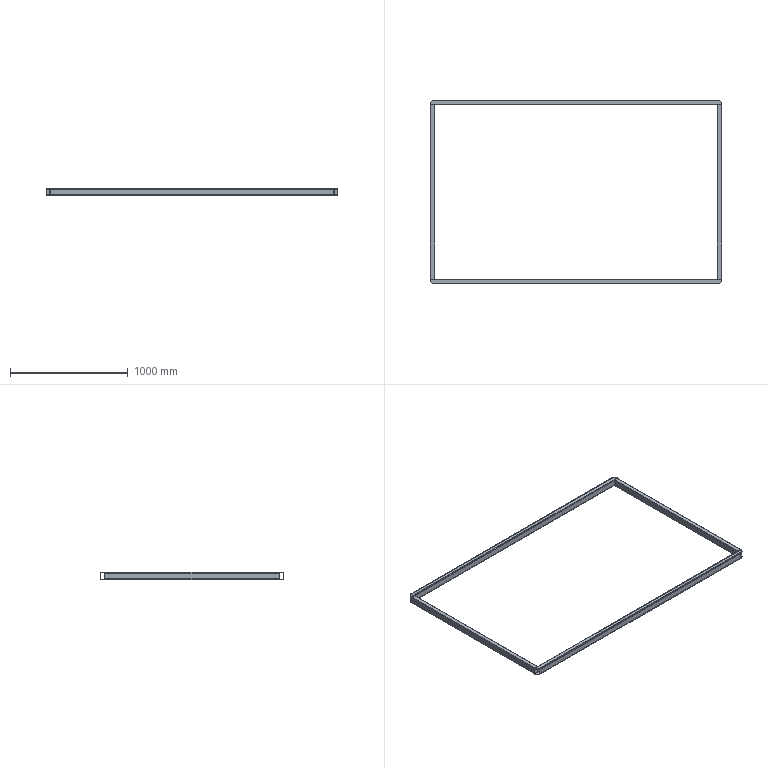Part | SolidWorks | features 3DProfileFeature 1, ICE 1, WeldMemberFeat 1, WeldmentFeature 1 | 4 solids | 72 faces | box 2480 x 1560 x 60 mm | volume 4257292 mm3 | plane 36 | cylinder 36 | commonest cylinder face diameters 6 x16 12 x16 80 x4